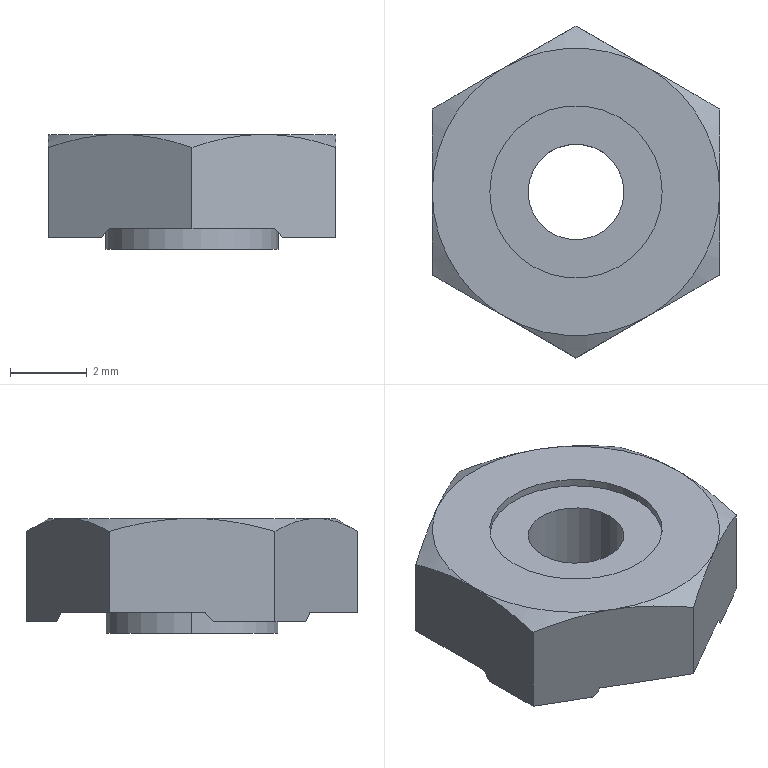Part | STEP file | Hex weld nut M3_DIN 929-M3-N | 1 solid | 32 faces | box 7.5 x 8.66 x 3 mm | volume 111.431 mm3 | plane 16 | cylinder 8 | cone 8 | commonest cylinder face diameters 4.5 x4 2.5 x2 3 x2